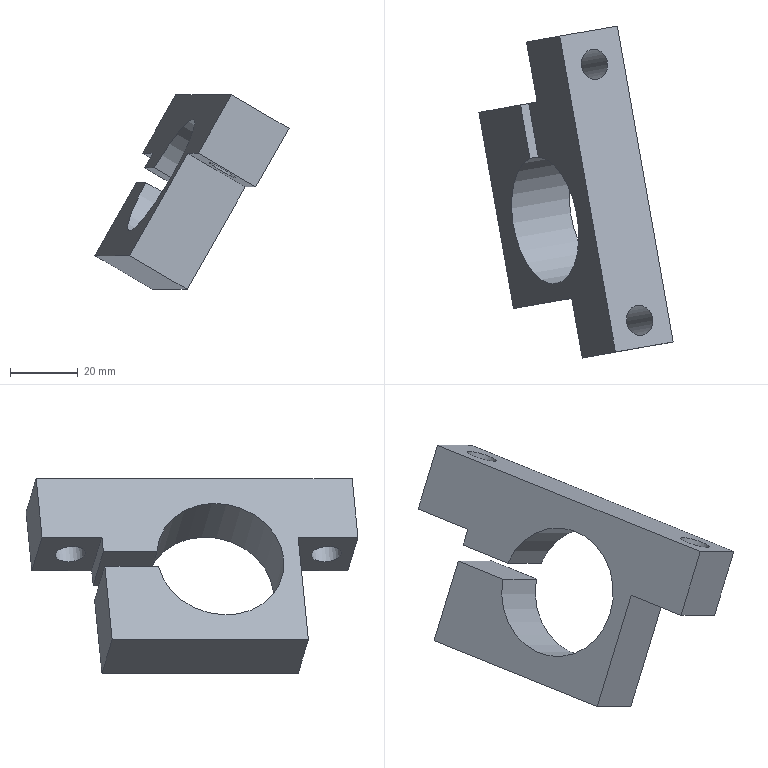Part | NX | features solid 2 | 1 solid | 16 faces | box 57.51 x 98.301 x 57.631 mm | volume 52353 mm3 | plane 13 | cylinder 3 | commonest cylinder face diameters 9 x2 38.1 x1
STEP:
#1=CARTESIAN_POINT('',(1020.919,60.813,-30.302));
#2=VERTEX_POINT('',#1);
#3=CARTESIAN_POINT('',(1037.976,63.82,-40.302));
#4=VERTEX_POINT('',#3);
#5=CARTESIAN_POINT('',(1037.976,63.82,-40.302));
#6=DIRECTION('',(0.8529,0.1504,-0.5));
#7=VECTOR('',#6,1000.);
#8=LINE('',#5,#7);
#9=EDGE_CURVE('',#2,#4,#8,.T.);
#10=ORIENTED_EDGE('',*,*,#9,.T.);
#11=CARTESIAN_POINT('',(1025.666,61.65,-61.953));
#12=VERTEX_POINT('',#11);
#13=CARTESIAN_POINT('',(1047.824,65.557,-22.982));
#14=DIRECTION('',(-0.4924,-0.08682,-0.866));
#15=VECTOR('',#14,1000.);
#16=LINE('',#13,#15);
#17=EDGE_CURVE('',#4,#12,#16,.T.);
#18=ORIENTED_EDGE('',*,*,#17,.T.);
#19=CARTESIAN_POINT('',(1008.609,58.642,-51.953));
#20=VERTEX_POINT('',#19);
#21=CARTESIAN_POINT('',(1025.666,61.65,-61.953));
#22=DIRECTION('',(-0.8529,-0.1504,0.5));
#23=VECTOR('',#22,1000.);
#24=LINE('',#21,#23);
#25=EDGE_CURVE('',#12,#20,#24,.T.);
#26=ORIENTED_EDGE('',*,*,#25,.T.);
#27=CARTESIAN_POINT('',(1030.767,62.549,-12.982));
#28=DIRECTION('',(-0.4924,-0.08682,-0.866));
#29=VECTOR('',#28,1000.);
#30=LINE('',#27,#29);
#31=EDGE_CURVE('',#2,#20,#30,.T.);
#32=ORIENTED_EDGE('',*,*,#31,.F.);
#33=EDGE_LOOP('',(#10,#18,#26,#32));
#34=FACE_BOUND('',#33,.T.);
#35=CARTESIAN_POINT('',(1047.824,65.557,-22.982));
#36=DIRECTION('',(0.1736,-0.9848,0.));
#37=DIRECTION('',(0.4924,0.08682,0.866));
#38=AXIS2_PLACEMENT_3D('',#35,#36,#37);
#39=PLANE('',#38);
#40=ADVANCED_FACE('',(#34),#39,.F.);
#41=ORIENTED_EDGE('',*,*,#25,.F.);
#42=CARTESIAN_POINT('',(1035.911,3.546,-61.953));
#43=VERTEX_POINT('',#42);
#44=CARTESIAN_POINT('',(1026.447,57.218,-61.953));
#45=DIRECTION('',(0.1736,-0.9848,0.));
#46=VECTOR('',#45,1000.);
#47=LINE('',#44,#46);
#48=EDGE_CURVE('',#12,#43,#47,.T.);
#49=ORIENTED_EDGE('',*,*,#48,.T.);
#50=CARTESIAN_POINT('',(1018.854,0.5386,-51.953));
#51=VERTEX_POINT('',#50);
#52=CARTESIAN_POINT('',(1035.911,3.546,-61.953));
#53=DIRECTION('',(-0.8529,-0.1504,0.5));
#54=VECTOR('',#53,1000.);
#55=LINE('',#52,#54);
#56=EDGE_CURVE('',#43,#51,#55,.T.);
#57=ORIENTED_EDGE('',*,*,#56,.T.);
#58=CARTESIAN_POINT('',(1009.39,54.211,-51.953));
#59=DIRECTION('',(0.1736,-0.9848,0.));
#60=VECTOR('',#59,1000.);
#61=LINE('',#58,#60);
#62=EDGE_CURVE('',#20,#51,#61,.T.);
#63=ORIENTED_EDGE('',*,*,#62,.F.);
#64=EDGE_LOOP('',(#41,#49,#57,#63));
#65=FACE_BOUND('',#64,.T.);
#66=CARTESIAN_POINT('',(1026.447,57.218,-61.953));
#67=DIRECTION('',(0.4924,0.08682,0.866));
#68=DIRECTION('',(-0.1736,0.9848,0.));
#69=AXIS2_PLACEMENT_3D('',#66,#67,#68);
#70=PLANE('',#69);
#71=ADVANCED_FACE('',(#65),#70,.F.);
#72=CARTESIAN_POINT('',(1025.843,61.681,-21.642));
#73=VERTEX_POINT('',#72);
#74=CARTESIAN_POINT('',(1023.381,61.247,-25.972));
#75=VERTEX_POINT('',#74);
#76=CARTESIAN_POINT('',(1030.767,62.549,-12.982));
#77=DIRECTION('',(-0.4924,-0.08682,-0.866));
#78=VECTOR('',#77,1000.);
#79=LINE('',#76,#78);
#80=EDGE_CURVE('',#73,#75,#79,.T.);
#81=ORIENTED_EDGE('',*,*,#80,.F.);
#82=CARTESIAN_POINT('',(1042.9,64.689,-31.642));
#83=VERTEX_POINT('',#82);
#84=CARTESIAN_POINT('',(1042.9,64.689,-31.642));
#85=DIRECTION('',(-0.8529,-0.1504,0.5));
#86=VECTOR('',#85,1000.);
#87=LINE('',#84,#86);
#88=EDGE_CURVE('',#83,#73,#87,.T.);
#89=ORIENTED_EDGE('',*,*,#88,.F.);
#90=CARTESIAN_POINT('',(1040.438,64.255,-35.972));
#91=VERTEX_POINT('',#90);
#92=CARTESIAN_POINT('',(1047.824,65.557,-22.982));
#93=DIRECTION('',(-0.4924,-0.08682,-0.866));
#94=VECTOR('',#93,1000.);
#95=LINE('',#92,#94);
#96=EDGE_CURVE('',#83,#91,#95,.T.);
#97=ORIENTED_EDGE('',*,*,#96,.T.);
#98=CARTESIAN_POINT('',(1040.438,64.255,-35.972));
#99=DIRECTION('',(0.8529,0.1504,-0.5));
#100=VECTOR('',#99,1000.);
#101=LINE('',#98,#100);
#102=EDGE_CURVE('',#75,#91,#101,.T.);
#103=ORIENTED_EDGE('',*,*,#102,.F.);
#104=EDGE_LOOP('',(#81,#89,#97,#103));
#105=FACE_BOUND('',#104,.T.);
#106=CARTESIAN_POINT('',(1047.824,65.557,-22.982));
#107=DIRECTION('',(0.1736,-0.9848,0.));
#108=DIRECTION('',(0.4924,0.08682,0.866));
#109=AXIS2_PLACEMENT_3D('',#106,#107,#108);
#110=PLANE('',#109);
#111=ADVANCED_FACE('',(#105),#110,.F.);
#112=CARTESIAN_POINT('',(1053.145,6.585,-31.642));
#113=VERTEX_POINT('',#112);
#114=CARTESIAN_POINT('',(1036.088,3.577,-21.642));
#115=VERTEX_POINT('',#114);
#116=CARTESIAN_POINT('',(1053.145,6.585,-31.642));
#117=DIRECTION('',(-0.8529,-0.1504,0.5));
#118=VECTOR('',#117,1000.);
#119=LINE('',#116,#118);
#120=EDGE_CURVE('',#113,#115,#119,.T.);
#121=ORIENTED_EDGE('',*,*,#120,.T.);
#122=CARTESIAN_POINT('',(1041.012,4.446,-12.982));
#123=DIRECTION('',(-0.4924,-0.08682,-0.866));
#124=VECTOR('',#123,1000.);
#125=LINE('',#122,#124);
#126=EDGE_CURVE('',#115,#51,#125,.T.);
#127=ORIENTED_EDGE('',*,*,#126,.T.);
#128=ORIENTED_EDGE('',*,*,#56,.F.);
#129=CARTESIAN_POINT('',(1058.069,7.453,-22.982));
#130=DIRECTION('',(-0.4924,-0.08682,-0.866));
#131=VECTOR('',#130,1000.);
#132=LINE('',#129,#131);
#133=EDGE_CURVE('',#113,#43,#132,.T.);
#134=ORIENTED_EDGE('',*,*,#133,.F.);
#135=EDGE_LOOP('',(#121,#127,#128,#134));
#136=FACE_BOUND('',#135,.T.);
#137=CARTESIAN_POINT('',(1058.069,7.453,-22.982));
#138=DIRECTION('',(0.1736,-0.9848,0.));
#139=DIRECTION('',(0.4924,0.08682,0.866));
#140=AXIS2_PLACEMENT_3D('',#137,#138,#139);
#141=PLANE('',#140);
#142=ADVANCED_FACE('',(#136),#141,.T.);
#143=CARTESIAN_POINT('',(1060.113,-3.03,-11.546));
#144=VERTEX_POINT('',#143);
#145=CARTESIAN_POINT('',(1056.201,-3.03,-9.321));
#146=DIRECTION('',(0.4924,0.08682,0.866));
#147=DIRECTION('',(0.8693,0.,-0.4943));
#148=AXIS2_PLACEMENT_3D('',#145,#146,#147);
#149=CIRCLE('',#148,4.5);
#150=EDGE_CURVE('',#144,#144,#149,.T.);
#151=ORIENTED_EDGE('',*,*,#150,.F.);
#152=EDGE_LOOP('',(#151));
#153=FACE_BOUND('',#152,.T.);
#154=CARTESIAN_POINT('',(1046.742,72.8,-11.546));
#155=VERTEX_POINT('',#154);
#156=CARTESIAN_POINT('',(1042.83,72.8,-9.321));
#157=DIRECTION('',(0.4924,0.08682,0.866));
#158=DIRECTION('',(0.8693,0.,-0.4943));
#159=AXIS2_PLACEMENT_3D('',#156,#157,#158);
#160=CIRCLE('',#159,4.5);
#161=EDGE_CURVE('',#155,#155,#160,.T.);
#162=ORIENTED_EDGE('',*,*,#161,.F.);
#163=EDGE_LOOP('',(#162));
#164=FACE_BOUND('',#163,.T.);
#165=CARTESIAN_POINT('',(1066.119,-9.405,-14.321));
#166=VERTEX_POINT('',#165);
#167=CARTESIAN_POINT('',(1049.062,-12.413,-4.321));
#168=VERTEX_POINT('',#167);
#169=CARTESIAN_POINT('',(1066.119,-9.405,-14.321));
#170=DIRECTION('',(0.8529,0.1504,-0.5));
#171=VECTOR('',#170,1000.);
#172=LINE('',#169,#171);
#173=EDGE_CURVE('',#166,#168,#172,.F.);
#174=ORIENTED_EDGE('',*,*,#173,.F.);
#175=CARTESIAN_POINT('',(1049.622,84.152,-14.321));
#176=VERTEX_POINT('',#175);
#177=CARTESIAN_POINT('',(1053.53,61.994,-14.321));
#178=DIRECTION('',(0.1736,-0.9848,0.));
#179=VECTOR('',#178,1000.);
#180=LINE('',#177,#179);
#181=EDGE_CURVE('',#176,#166,#180,.T.);
#182=ORIENTED_EDGE('',*,*,#181,.F.);
#183=CARTESIAN_POINT('',(1032.565,81.144,-4.321));
#184=VERTEX_POINT('',#183);
#185=CARTESIAN_POINT('',(1049.622,84.152,-14.321));
#186=DIRECTION('',(-0.8529,-0.1504,0.5));
#187=VECTOR('',#186,1000.);
#188=LINE('',#185,#187);
#189=EDGE_CURVE('',#176,#184,#188,.T.);
#190=ORIENTED_EDGE('',*,*,#189,.T.);
#191=CARTESIAN_POINT('',(1036.472,58.986,-4.321));
#192=DIRECTION('',(0.1736,-0.9848,0.));
#193=VECTOR('',#192,1000.);
#194=LINE('',#191,#193);
#195=EDGE_CURVE('',#184,#168,#194,.T.);
#196=ORIENTED_EDGE('',*,*,#195,.T.);
#197=EDGE_LOOP('',(#174,#182,#190,#196));
#198=FACE_BOUND('',#197,.T.);
#199=CARTESIAN_POINT('',(1053.53,61.994,-14.321));
#200=DIRECTION('',(0.4924,0.08682,0.866));
#201=DIRECTION('',(-0.1736,0.9848,0.));
#202=AXIS2_PLACEMENT_3D('',#199,#200,#201);
#203=PLANE('',#202);
#204=ADVANCED_FACE('',(#153,#164,#198),#203,.T.);
#205=CARTESIAN_POINT('',(1043.236,48.385,-35.972));
#206=VERTEX_POINT('',#205);
#207=CARTESIAN_POINT('',(1041.219,59.823,-35.972));
#208=DIRECTION('',(-0.1736,0.9848,0.));
#209=VECTOR('',#208,1000.);
#210=LINE('',#207,#209);
#211=EDGE_CURVE('',#206,#91,#210,.T.);
#212=ORIENTED_EDGE('',*,*,#211,.T.);
#213=ORIENTED_EDGE('',*,*,#96,.F.);
#214=CARTESIAN_POINT('',(1039.774,82.415,-31.642));
#215=VERTEX_POINT('',#214);
#216=CARTESIAN_POINT('',(1043.681,60.257,-31.642));
#217=DIRECTION('',(-0.1736,0.9848,0.));
#218=VECTOR('',#217,1000.);
#219=LINE('',#216,#218);
#220=EDGE_CURVE('',#83,#215,#219,.T.);
#221=ORIENTED_EDGE('',*,*,#220,.T.);
#222=CARTESIAN_POINT('',(1044.698,83.284,-22.982));
#223=DIRECTION('',(-0.4924,-0.08682,-0.866));
#224=VECTOR('',#223,1000.);
#225=LINE('',#222,#224);
#226=EDGE_CURVE('',#176,#215,#225,.T.);
#227=ORIENTED_EDGE('',*,*,#226,.F.);
#228=ORIENTED_EDGE('',*,*,#181,.T.);
#229=CARTESIAN_POINT('',(1056.271,-11.141,-31.642));
#230=VERTEX_POINT('',#229);
#231=CARTESIAN_POINT('',(1035.59,-14.788,-68.015));
#232=DIRECTION('',(0.4924,0.08682,0.866));
#233=VECTOR('',#232,1000.);
#234=LINE('',#231,#233);
#235=EDGE_CURVE('',#166,#230,#234,.F.);
#236=ORIENTED_EDGE('',*,*,#235,.T.);
#237=CARTESIAN_POINT('',(1043.681,60.257,-31.642));
#238=DIRECTION('',(-0.1736,0.9848,0.));
#239=VECTOR('',#238,1000.);
#240=LINE('',#237,#239);
#241=EDGE_CURVE('',#230,#113,#240,.T.);
#242=ORIENTED_EDGE('',*,*,#241,.T.);
#243=ORIENTED_EDGE('',*,*,#133,.T.);
#244=ORIENTED_EDGE('',*,*,#48,.F.);
#245=ORIENTED_EDGE('',*,*,#17,.F.);
#246=CARTESIAN_POINT('',(1040.774,47.951,-40.302));
#247=VERTEX_POINT('',#246);
#248=CARTESIAN_POINT('',(1038.757,59.389,-40.302));
#249=DIRECTION('',(-0.1736,0.9848,0.));
#250=VECTOR('',#249,1000.);
#251=LINE('',#248,#250);
#252=EDGE_CURVE('',#247,#4,#251,.T.);
#253=ORIENTED_EDGE('',*,*,#252,.F.);
#254=CARTESIAN_POINT('',(1045.285,29.569,-38.137));
#255=DIRECTION('',(0.8529,0.1504,-0.5));
#256=DIRECTION('',(0.4924,0.08682,0.866));
#257=AXIS2_PLACEMENT_3D('',#254,#255,#256);
#258=CIRCLE('',#257,19.05);
#259=EDGE_CURVE('',#206,#247,#258,.T.);
#260=ORIENTED_EDGE('',*,*,#259,.F.);
#261=EDGE_LOOP('',(#212,#213,#221,#227,#228,#236,#242,#243,#244,#245,#253,#260));
#262=FACE_BOUND('',#261,.T.);
#263=CARTESIAN_POINT('',(1023.001,56.61,-68.015));
#264=DIRECTION('',(0.8529,0.1504,-0.5));
#265=DIRECTION('',(0.4924,0.08682,0.866));
#266=AXIS2_PLACEMENT_3D('',#263,#264,#265);
#267=PLANE('',#266);
#268=ADVANCED_FACE('',(#262),#267,.T.);
#269=CARTESIAN_POINT('',(1023.717,44.943,-30.302));
#270=VERTEX_POINT('',#269);
#271=CARTESIAN_POINT('',(1026.179,45.377,-25.972));
#272=VERTEX_POINT('',#271);
#273=CARTESIAN_POINT('',(1028.227,26.562,-28.137));
#274=DIRECTION('',(-0.8529,-0.1504,0.5));
#275=DIRECTION('',(-0.4924,-0.08682,-0.866));
#276=AXIS2_PLACEMENT_3D('',#273,#274,#275);
#277=CIRCLE('',#276,19.05);
#278=EDGE_CURVE('',#270,#272,#277,.T.);
#279=ORIENTED_EDGE('',*,*,#278,.F.);
#280=CARTESIAN_POINT('',(1021.7,56.381,-30.302));
#281=DIRECTION('',(-0.1736,0.9848,0.));
#282=VECTOR('',#281,1000.);
#283=LINE('',#280,#282);
#284=EDGE_CURVE('',#270,#2,#283,.T.);
#285=ORIENTED_EDGE('',*,*,#284,.T.);
#286=ORIENTED_EDGE('',*,*,#31,.T.);
#287=ORIENTED_EDGE('',*,*,#62,.T.);
#288=ORIENTED_EDGE('',*,*,#126,.F.);
#289=CARTESIAN_POINT('',(1039.214,-14.149,-21.642));
#290=VERTEX_POINT('',#289);
#291=CARTESIAN_POINT('',(1026.624,57.249,-21.642));
#292=DIRECTION('',(-0.1736,0.9848,0.));
#293=VECTOR('',#292,1000.);
#294=LINE('',#291,#293);
#295=EDGE_CURVE('',#290,#115,#294,.T.);
#296=ORIENTED_EDGE('',*,*,#295,.F.);
#297=CARTESIAN_POINT('',(1018.533,-17.796,-58.015));
#298=DIRECTION('',(0.4924,0.08682,0.866));
#299=VECTOR('',#298,1000.);
#300=LINE('',#297,#299);
#301=EDGE_CURVE('',#168,#290,#300,.F.);
#302=ORIENTED_EDGE('',*,*,#301,.F.);
#303=ORIENTED_EDGE('',*,*,#195,.F.);
#304=CARTESIAN_POINT('',(1022.717,79.408,-21.642));
#305=VERTEX_POINT('',#304);
#306=CARTESIAN_POINT('',(1027.641,80.276,-12.982));
#307=DIRECTION('',(-0.4924,-0.08682,-0.866));
#308=VECTOR('',#307,1000.);
#309=LINE('',#306,#308);
#310=EDGE_CURVE('',#184,#305,#309,.T.);
#311=ORIENTED_EDGE('',*,*,#310,.T.);
#312=CARTESIAN_POINT('',(1026.624,57.249,-21.642));
#313=DIRECTION('',(-0.1736,0.9848,0.));
#314=VECTOR('',#313,1000.);
#315=LINE('',#312,#314);
#316=EDGE_CURVE('',#73,#305,#315,.T.);
#317=ORIENTED_EDGE('',*,*,#316,.F.);
#318=ORIENTED_EDGE('',*,*,#80,.T.);
#319=CARTESIAN_POINT('',(1024.162,56.815,-25.972));
#320=DIRECTION('',(-0.1736,0.9848,0.));
#321=VECTOR('',#320,1000.);
#322=LINE('',#319,#321);
#323=EDGE_CURVE('',#272,#75,#322,.T.);
#324=ORIENTED_EDGE('',*,*,#323,.F.);
#325=EDGE_LOOP('',(#279,#285,#286,#287,#288,#296,#302,#303,#311,#317,#318,#324));
#326=FACE_BOUND('',#325,.T.);
#327=CARTESIAN_POINT('',(1005.943,53.603,-58.015));
#328=DIRECTION('',(0.8529,0.1504,-0.5));
#329=DIRECTION('',(0.4924,0.08682,0.866));
#330=AXIS2_PLACEMENT_3D('',#327,#328,#329);
#331=PLANE('',#330);
#332=ADVANCED_FACE('',(#326),#331,.F.);
#333=ORIENTED_EDGE('',*,*,#310,.F.);
#334=ORIENTED_EDGE('',*,*,#189,.F.);
#335=ORIENTED_EDGE('',*,*,#226,.T.);
#336=CARTESIAN_POINT('',(1039.774,82.415,-31.642));
#337=DIRECTION('',(-0.8529,-0.1504,0.5));
#338=VECTOR('',#337,1000.);
#339=LINE('',#336,#338);
#340=EDGE_CURVE('',#215,#305,#339,.T.);
#341=ORIENTED_EDGE('',*,*,#340,.T.);
#342=EDGE_LOOP('',(#333,#334,#335,#341));
#343=FACE_BOUND('',#342,.T.);
#344=CARTESIAN_POINT('',(1044.698,83.284,-22.982));
#345=DIRECTION('',(0.1736,-0.9848,0.));
#346=DIRECTION('',(-0.8529,-0.1504,0.5));
#347=AXIS2_PLACEMENT_3D('',#344,#345,#346);
#348=PLANE('',#347);
#349=ADVANCED_FACE('',(#343),#348,.F.);
#350=CARTESIAN_POINT('',(1036.894,71.063,-28.866));
#351=VERTEX_POINT('',#350);
#352=CARTESIAN_POINT('',(1032.982,71.063,-26.642));
#353=DIRECTION('',(0.4924,0.08682,0.866));
#354=DIRECTION('',(0.8693,0.,-0.4943));
#355=AXIS2_PLACEMENT_3D('',#352,#353,#354);
#356=CIRCLE('',#355,4.5);
#357=EDGE_CURVE('',#351,#351,#356,.T.);
#358=ORIENTED_EDGE('',*,*,#357,.T.);
#359=EDGE_LOOP('',(#358));
#360=FACE_BOUND('',#359,.T.);
#361=ORIENTED_EDGE('',*,*,#340,.F.);
#362=ORIENTED_EDGE('',*,*,#220,.F.);
#363=ORIENTED_EDGE('',*,*,#88,.T.);
#364=ORIENTED_EDGE('',*,*,#316,.T.);
#365=EDGE_LOOP('',(#361,#362,#363,#364));
#366=FACE_BOUND('',#365,.T.);
#367=CARTESIAN_POINT('',(1043.681,60.257,-31.642));
#368=DIRECTION('',(0.4924,0.08682,0.866));
#369=DIRECTION('',(0.8529,0.1504,-0.5));
#370=AXIS2_PLACEMENT_3D('',#367,#368,#369);
#371=PLANE('',#370);
#372=ADVANCED_FACE('',(#360,#366),#371,.F.);
#373=ORIENTED_EDGE('',*,*,#235,.F.);
#374=ORIENTED_EDGE('',*,*,#173,.T.);
#375=ORIENTED_EDGE('',*,*,#301,.T.);
#376=CARTESIAN_POINT('',(1056.271,-11.141,-31.642));
#377=DIRECTION('',(0.8529,0.1504,-0.5));
#378=VECTOR('',#377,1000.);
#379=LINE('',#376,#378);
#380=EDGE_CURVE('',#230,#290,#379,.F.);
#381=ORIENTED_EDGE('',*,*,#380,.F.);
#382=EDGE_LOOP('',(#373,#374,#375,#381));
#383=FACE_BOUND('',#382,.T.);
#384=CARTESIAN_POINT('',(1061.195,-10.273,-22.982));
#385=DIRECTION('',(0.1736,-0.9848,0.));
#386=DIRECTION('',(-0.8529,-0.1504,0.5));
#387=AXIS2_PLACEMENT_3D('',#384,#385,#386);
#388=PLANE('',#387);
#389=ADVANCED_FACE('',(#383),#388,.T.);
#390=CARTESIAN_POINT('',(1050.265,-4.767,-28.866));
#391=VERTEX_POINT('',#390);
#392=CARTESIAN_POINT('',(1046.353,-4.767,-26.642));
#393=DIRECTION('',(0.4924,0.08682,0.866));
#394=DIRECTION('',(0.8693,0.,-0.4943));
#395=AXIS2_PLACEMENT_3D('',#392,#393,#394);
#396=CIRCLE('',#395,4.5);
#397=EDGE_CURVE('',#391,#391,#396,.T.);
#398=ORIENTED_EDGE('',*,*,#397,.T.);
#399=EDGE_LOOP('',(#398));
#400=FACE_BOUND('',#399,.T.);
#401=ORIENTED_EDGE('',*,*,#120,.F.);
#402=ORIENTED_EDGE('',*,*,#241,.F.);
#403=ORIENTED_EDGE('',*,*,#380,.T.);
#404=ORIENTED_EDGE('',*,*,#295,.T.);
#405=EDGE_LOOP('',(#401,#402,#403,#404));
#406=FACE_BOUND('',#405,.T.);
#407=CARTESIAN_POINT('',(1055.49,-6.71,-31.642));
#408=DIRECTION('',(0.4924,0.08682,0.866));
#409=DIRECTION('',(0.8529,0.1504,-0.5));
#410=AXIS2_PLACEMENT_3D('',#407,#408,#409);
#411=PLANE('',#410);
#412=ADVANCED_FACE('',(#400,#406),#411,.F.);
#413=ORIENTED_EDGE('',*,*,#259,.T.);
#414=CARTESIAN_POINT('',(1040.774,47.951,-40.302));
#415=DIRECTION('',(-0.8529,-0.1504,0.5));
#416=VECTOR('',#415,1000.);
#417=LINE('',#414,#416);
#418=EDGE_CURVE('',#247,#270,#417,.T.);
#419=ORIENTED_EDGE('',*,*,#418,.T.);
#420=ORIENTED_EDGE('',*,*,#278,.T.);
#421=CARTESIAN_POINT('',(1043.236,48.385,-35.972));
#422=DIRECTION('',(-0.8529,-0.1504,0.5));
#423=VECTOR('',#422,1000.);
#424=LINE('',#421,#423);
#425=EDGE_CURVE('',#206,#272,#424,.T.);
#426=ORIENTED_EDGE('',*,*,#425,.F.);
#427=EDGE_LOOP('',(#413,#419,#420,#426));
#428=FACE_BOUND('',#427,.T.);
#429=CARTESIAN_POINT('',(1045.285,29.569,-38.137));
#430=DIRECTION('',(-0.8529,-0.1504,0.5));
#431=DIRECTION('',(0.4924,0.08682,0.866));
#432=AXIS2_PLACEMENT_3D('',#429,#430,#431);
#433=CYLINDRICAL_SURFACE('',#432,19.05);
#434=ADVANCED_FACE('',(#428),#433,.F.);
#435=ORIENTED_EDGE('',*,*,#9,.F.);
#436=ORIENTED_EDGE('',*,*,#284,.F.);
#437=ORIENTED_EDGE('',*,*,#418,.F.);
#438=ORIENTED_EDGE('',*,*,#252,.T.);
#439=EDGE_LOOP('',(#435,#436,#437,#438));
#440=FACE_BOUND('',#439,.T.);
#441=CARTESIAN_POINT('',(958.767,14.314,9.698));
#442=DIRECTION('',(0.4924,0.08682,0.866));
#443=DIRECTION('',(0.8529,0.1504,-0.5));
#444=AXIS2_PLACEMENT_3D('',#441,#442,#443);
#445=PLANE('',#444);
#446=ADVANCED_FACE('',(#440),#445,.T.);
#447=ORIENTED_EDGE('',*,*,#323,.T.);
#448=ORIENTED_EDGE('',*,*,#102,.T.);
#449=ORIENTED_EDGE('',*,*,#211,.F.);
#450=ORIENTED_EDGE('',*,*,#425,.T.);
#451=EDGE_LOOP('',(#447,#448,#449,#450));
#452=FACE_BOUND('',#451,.T.);
#453=CARTESIAN_POINT('',(961.229,14.748,14.028));
#454=DIRECTION('',(0.4924,0.08682,0.866));
#455=DIRECTION('',(0.8529,0.1504,-0.5));
#456=AXIS2_PLACEMENT_3D('',#453,#454,#455);
#457=PLANE('',#456);
#458=ADVANCED_FACE('',(#452),#457,.F.);
#459=ORIENTED_EDGE('',*,*,#161,.T.);
#460=EDGE_LOOP('',(#459));
#461=FACE_BOUND('',#460,.T.);
#462=ORIENTED_EDGE('',*,*,#357,.F.);
#463=EDGE_LOOP('',(#462));
#464=FACE_BOUND('',#463,.T.);
#465=CARTESIAN_POINT('',(1032.982,71.063,-26.642));
#466=DIRECTION('',(0.4924,0.08682,0.866));
#467=DIRECTION('',(0.8693,0.,-0.4943));
#468=AXIS2_PLACEMENT_3D('',#465,#466,#467);
#469=CYLINDRICAL_SURFACE('',#468,4.5);
#470=ADVANCED_FACE('',(#461,#464),#469,.F.);
#471=ORIENTED_EDGE('',*,*,#150,.T.);
#472=EDGE_LOOP('',(#471));
#473=FACE_BOUND('',#472,.T.);
#474=ORIENTED_EDGE('',*,*,#397,.F.);
#475=EDGE_LOOP('',(#474));
#476=FACE_BOUND('',#475,.T.);
#477=CARTESIAN_POINT('',(1046.353,-4.767,-26.642));
#478=DIRECTION('',(0.4924,0.08682,0.866));
#479=DIRECTION('',(0.8693,0.,-0.4943));
#480=AXIS2_PLACEMENT_3D('',#477,#478,#479);
#481=CYLINDRICAL_SURFACE('',#480,4.5);
#482=ADVANCED_FACE('',(#473,#476),#481,.F.);
#483=CLOSED_SHELL('',(#40,#71,#111,#142,#204,#268,#332,#349,#372,#389,#412,#434,#446,#458,#470,#482));
#484=MANIFOLD_SOLID_BREP('',#483);
#485=(LENGTH_UNIT()NAMED_UNIT(*)SI_UNIT(.MILLI.,.METRE.));
#486=UNCERTAINTY_MEASURE_WITH_UNIT(LENGTH_MEASURE(0.00001),#485,'','');
#487=(NAMED_UNIT(*)PLANE_ANGLE_UNIT()SI_UNIT($,.RADIAN.));
#488=(NAMED_UNIT(*)SI_UNIT($,.STERADIAN.)SOLID_ANGLE_UNIT());
#489=(GEOMETRIC_REPRESENTATION_CONTEXT(3)GLOBAL_UNCERTAINTY_ASSIGNED_CONTEXT((#486))GLOBAL_UNIT_ASSIGNED_CONTEXT((#485,#487,#488))REPRESENTATION_CONTEXT('',''));
#490=ADVANCED_BREP_SHAPE_REPRESENTATION('',(#484),#489);